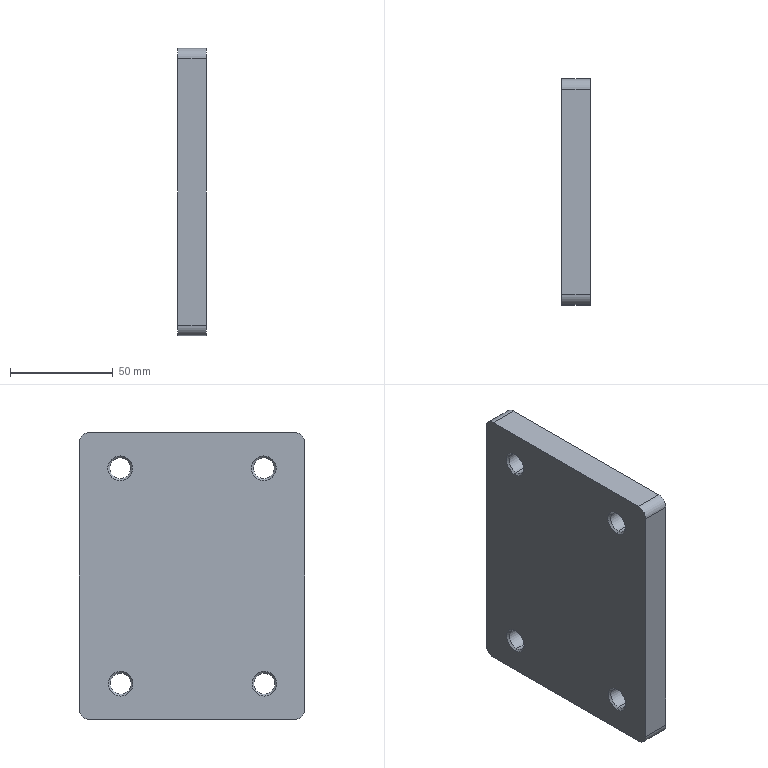Part | SolidWorks | features Extrusion 1, Fillet 1, HoleWzd 1 | 1 solid | 26 faces | box 14 x 110 x 140 mm | volume 210665 mm3 | cylinder 12 | cone 8 | plane 6 | commonest cylinder face diameters 10.2 x8 10 x4
STEP:
#1=CARTESIAN_POINT('',(0.925,34.757,-57.6));
#2=VERTEX_POINT('',#1);
#3=CARTESIAN_POINT('',(0.925,34.757,-47.4));
#4=VERTEX_POINT('',#3);
#5=CARTESIAN_POINT('',(0.925,34.757,-52.5));
#6=DIRECTION('',(-1.,0.,0.));
#7=DIRECTION('',(0.,0.,1.));
#8=AXIS2_PLACEMENT_3D('',#5,#6,#7);
#9=CIRCLE('',#8,5.1);
#10=EDGE_CURVE('',#2,#4,#9,.T.);
#11=ORIENTED_EDGE('',*,*,#10,.F.);
#12=CARTESIAN_POINT('',(0.,34.757,-58.525));
#13=VERTEX_POINT('',#12);
#14=CARTESIAN_POINT('',(0.,34.757,-58.525));
#15=DIRECTION('',(-0.7071,0.,-0.7071));
#16=VECTOR('',#15,1000.);
#17=LINE('',#14,#16);
#18=EDGE_CURVE('',#2,#13,#17,.T.);
#19=ORIENTED_EDGE('',*,*,#18,.T.);
#20=CARTESIAN_POINT('',(0.,34.757,-46.475));
#21=VERTEX_POINT('',#20);
#22=CARTESIAN_POINT('',(0.,34.757,-52.5));
#23=DIRECTION('',(-1.,0.,0.));
#24=DIRECTION('',(0.,0.,1.));
#25=AXIS2_PLACEMENT_3D('',#22,#23,#24);
#26=CIRCLE('',#25,6.025);
#27=EDGE_CURVE('',#13,#21,#26,.T.);
#28=ORIENTED_EDGE('',*,*,#27,.T.);
#29=CARTESIAN_POINT('',(0.,34.757,-46.475));
#30=DIRECTION('',(-0.7071,0.,0.7071));
#31=VECTOR('',#30,1000.);
#32=LINE('',#29,#31);
#33=EDGE_CURVE('',#4,#21,#32,.T.);
#34=ORIENTED_EDGE('',*,*,#33,.F.);
#35=EDGE_LOOP('',(#11,#19,#28,#34));
#36=FACE_OUTER_BOUND('',#35,.T.);
#37=CARTESIAN_POINT('',(0.,34.757,-52.5));
#38=DIRECTION('',(-1.,0.,0.));
#39=DIRECTION('',(0.,0.,1.));
#40=AXIS2_PLACEMENT_3D('',#37,#38,#39);
#41=CONICAL_SURFACE('',#40,6.025,0.7854);
#42=ADVANCED_FACE('',(#36),#41,.F.);
#43=CARTESIAN_POINT('',(14.,34.757,-57.6));
#44=VERTEX_POINT('',#43);
#45=CARTESIAN_POINT('',(14.,34.757,-47.4));
#46=VERTEX_POINT('',#45);
#47=CARTESIAN_POINT('',(14.,34.757,-52.5));
#48=DIRECTION('',(-1.,0.,0.));
#49=DIRECTION('',(0.,0.,1.));
#50=AXIS2_PLACEMENT_3D('',#47,#48,#49);
#51=CIRCLE('',#50,5.1);
#52=EDGE_CURVE('',#44,#46,#51,.T.);
#53=ORIENTED_EDGE('',*,*,#52,.F.);
#54=CARTESIAN_POINT('',(0.,34.757,-57.6));
#55=DIRECTION('',(-1.,0.,0.));
#56=VECTOR('',#55,1000.);
#57=LINE('',#54,#56);
#58=EDGE_CURVE('',#44,#2,#57,.T.);
#59=ORIENTED_EDGE('',*,*,#58,.T.);
#60=ORIENTED_EDGE('',*,*,#10,.T.);
#61=CARTESIAN_POINT('',(0.,34.757,-47.4));
#62=DIRECTION('',(-1.,0.,0.));
#63=VECTOR('',#62,1000.);
#64=LINE('',#61,#63);
#65=EDGE_CURVE('',#46,#4,#64,.T.);
#66=ORIENTED_EDGE('',*,*,#65,.F.);
#67=EDGE_LOOP('',(#53,#59,#60,#66));
#68=FACE_OUTER_BOUND('',#67,.T.);
#69=CARTESIAN_POINT('',(0.,34.757,-52.5));
#70=DIRECTION('',(-1.,0.,0.));
#71=DIRECTION('',(0.,0.,1.));
#72=AXIS2_PLACEMENT_3D('',#69,#70,#71);
#73=CYLINDRICAL_SURFACE('',#72,5.1);
#74=ADVANCED_FACE('',(#68),#73,.F.);
#75=CARTESIAN_POINT('',(0.925,35.,47.4));
#76=VERTEX_POINT('',#75);
#77=CARTESIAN_POINT('',(0.925,35.,57.6));
#78=VERTEX_POINT('',#77);
#79=CARTESIAN_POINT('',(0.925,35.,52.5));
#80=DIRECTION('',(-1.,0.,0.));
#81=DIRECTION('',(0.,0.,1.));
#82=AXIS2_PLACEMENT_3D('',#79,#80,#81);
#83=CIRCLE('',#82,5.1);
#84=EDGE_CURVE('',#76,#78,#83,.T.);
#85=ORIENTED_EDGE('',*,*,#84,.F.);
#86=CARTESIAN_POINT('',(0.,35.,46.475));
#87=VERTEX_POINT('',#86);
#88=CARTESIAN_POINT('',(0.,35.,46.475));
#89=DIRECTION('',(-0.7071,0.,-0.7071));
#90=VECTOR('',#89,1000.);
#91=LINE('',#88,#90);
#92=EDGE_CURVE('',#76,#87,#91,.T.);
#93=ORIENTED_EDGE('',*,*,#92,.T.);
#94=CARTESIAN_POINT('',(0.,35.,58.525));
#95=VERTEX_POINT('',#94);
#96=CARTESIAN_POINT('',(0.,35.,52.5));
#97=DIRECTION('',(-1.,0.,0.));
#98=DIRECTION('',(0.,0.,1.));
#99=AXIS2_PLACEMENT_3D('',#96,#97,#98);
#100=CIRCLE('',#99,6.025);
#101=EDGE_CURVE('',#87,#95,#100,.T.);
#102=ORIENTED_EDGE('',*,*,#101,.T.);
#103=CARTESIAN_POINT('',(0.,35.,58.525));
#104=DIRECTION('',(-0.7071,0.,0.7071));
#105=VECTOR('',#104,1000.);
#106=LINE('',#103,#105);
#107=EDGE_CURVE('',#78,#95,#106,.T.);
#108=ORIENTED_EDGE('',*,*,#107,.F.);
#109=EDGE_LOOP('',(#85,#93,#102,#108));
#110=FACE_OUTER_BOUND('',#109,.T.);
#111=CARTESIAN_POINT('',(0.,35.,52.5));
#112=DIRECTION('',(-1.,0.,0.));
#113=DIRECTION('',(0.,0.,1.));
#114=AXIS2_PLACEMENT_3D('',#111,#112,#113);
#115=CONICAL_SURFACE('',#114,6.025,0.7854);
#116=ADVANCED_FACE('',(#110),#115,.F.);
#117=CARTESIAN_POINT('',(14.,35.,47.4));
#118=VERTEX_POINT('',#117);
#119=CARTESIAN_POINT('',(14.,35.,57.6));
#120=VERTEX_POINT('',#119);
#121=CARTESIAN_POINT('',(14.,35.,52.5));
#122=DIRECTION('',(-1.,0.,0.));
#123=DIRECTION('',(0.,0.,1.));
#124=AXIS2_PLACEMENT_3D('',#121,#122,#123);
#125=CIRCLE('',#124,5.1);
#126=EDGE_CURVE('',#118,#120,#125,.T.);
#127=ORIENTED_EDGE('',*,*,#126,.F.);
#128=CARTESIAN_POINT('',(0.,35.,47.4));
#129=DIRECTION('',(-1.,0.,0.));
#130=VECTOR('',#129,1000.);
#131=LINE('',#128,#130);
#132=EDGE_CURVE('',#118,#76,#131,.T.);
#133=ORIENTED_EDGE('',*,*,#132,.T.);
#134=ORIENTED_EDGE('',*,*,#84,.T.);
#135=CARTESIAN_POINT('',(0.,35.,57.6));
#136=DIRECTION('',(-1.,0.,0.));
#137=VECTOR('',#136,1000.);
#138=LINE('',#135,#137);
#139=EDGE_CURVE('',#120,#78,#138,.T.);
#140=ORIENTED_EDGE('',*,*,#139,.F.);
#141=EDGE_LOOP('',(#127,#133,#134,#140));
#142=FACE_OUTER_BOUND('',#141,.T.);
#143=CARTESIAN_POINT('',(0.,35.,52.5));
#144=DIRECTION('',(-1.,0.,0.));
#145=DIRECTION('',(0.,0.,1.));
#146=AXIS2_PLACEMENT_3D('',#143,#144,#145);
#147=CYLINDRICAL_SURFACE('',#146,5.1);
#148=ADVANCED_FACE('',(#142),#147,.F.);
#149=CARTESIAN_POINT('',(0.925,-35.,47.4));
#150=VERTEX_POINT('',#149);
#151=CARTESIAN_POINT('',(0.925,-35.,57.6));
#152=VERTEX_POINT('',#151);
#153=CARTESIAN_POINT('',(0.925,-35.,52.5));
#154=DIRECTION('',(-1.,0.,0.));
#155=DIRECTION('',(0.,0.,1.));
#156=AXIS2_PLACEMENT_3D('',#153,#154,#155);
#157=CIRCLE('',#156,5.1);
#158=EDGE_CURVE('',#150,#152,#157,.T.);
#159=ORIENTED_EDGE('',*,*,#158,.F.);
#160=CARTESIAN_POINT('',(0.,-35.,46.475));
#161=VERTEX_POINT('',#160);
#162=CARTESIAN_POINT('',(0.,-35.,46.475));
#163=DIRECTION('',(-0.7071,0.,-0.7071));
#164=VECTOR('',#163,1000.);
#165=LINE('',#162,#164);
#166=EDGE_CURVE('',#150,#161,#165,.T.);
#167=ORIENTED_EDGE('',*,*,#166,.T.);
#168=CARTESIAN_POINT('',(0.,-35.,58.525));
#169=VERTEX_POINT('',#168);
#170=CARTESIAN_POINT('',(0.,-35.,52.5));
#171=DIRECTION('',(-1.,0.,0.));
#172=DIRECTION('',(0.,0.,1.));
#173=AXIS2_PLACEMENT_3D('',#170,#171,#172);
#174=CIRCLE('',#173,6.025);
#175=EDGE_CURVE('',#161,#169,#174,.T.);
#176=ORIENTED_EDGE('',*,*,#175,.T.);
#177=CARTESIAN_POINT('',(0.,-35.,58.525));
#178=DIRECTION('',(-0.7071,0.,0.7071));
#179=VECTOR('',#178,1000.);
#180=LINE('',#177,#179);
#181=EDGE_CURVE('',#152,#169,#180,.T.);
#182=ORIENTED_EDGE('',*,*,#181,.F.);
#183=EDGE_LOOP('',(#159,#167,#176,#182));
#184=FACE_OUTER_BOUND('',#183,.T.);
#185=CARTESIAN_POINT('',(0.,-35.,52.5));
#186=DIRECTION('',(-1.,0.,0.));
#187=DIRECTION('',(0.,0.,1.));
#188=AXIS2_PLACEMENT_3D('',#185,#186,#187);
#189=CONICAL_SURFACE('',#188,6.025,0.7854);
#190=ADVANCED_FACE('',(#184),#189,.F.);
#191=CARTESIAN_POINT('',(14.,-35.,47.4));
#192=VERTEX_POINT('',#191);
#193=CARTESIAN_POINT('',(14.,-35.,57.6));
#194=VERTEX_POINT('',#193);
#195=CARTESIAN_POINT('',(14.,-35.,52.5));
#196=DIRECTION('',(-1.,0.,0.));
#197=DIRECTION('',(0.,0.,1.));
#198=AXIS2_PLACEMENT_3D('',#195,#196,#197);
#199=CIRCLE('',#198,5.1);
#200=EDGE_CURVE('',#192,#194,#199,.T.);
#201=ORIENTED_EDGE('',*,*,#200,.F.);
#202=CARTESIAN_POINT('',(0.,-35.,47.4));
#203=DIRECTION('',(-1.,0.,0.));
#204=VECTOR('',#203,1000.);
#205=LINE('',#202,#204);
#206=EDGE_CURVE('',#192,#150,#205,.T.);
#207=ORIENTED_EDGE('',*,*,#206,.T.);
#208=ORIENTED_EDGE('',*,*,#158,.T.);
#209=CARTESIAN_POINT('',(0.,-35.,57.6));
#210=DIRECTION('',(-1.,0.,0.));
#211=VECTOR('',#210,1000.);
#212=LINE('',#209,#211);
#213=EDGE_CURVE('',#194,#152,#212,.T.);
#214=ORIENTED_EDGE('',*,*,#213,.F.);
#215=EDGE_LOOP('',(#201,#207,#208,#214));
#216=FACE_OUTER_BOUND('',#215,.T.);
#217=CARTESIAN_POINT('',(0.,-35.,52.5));
#218=DIRECTION('',(-1.,0.,0.));
#219=DIRECTION('',(0.,0.,1.));
#220=AXIS2_PLACEMENT_3D('',#217,#218,#219);
#221=CYLINDRICAL_SURFACE('',#220,5.1);
#222=ADVANCED_FACE('',(#216),#221,.F.);
#223=CARTESIAN_POINT('',(0.925,-35.243,-57.6));
#224=VERTEX_POINT('',#223);
#225=CARTESIAN_POINT('',(0.925,-35.243,-47.4));
#226=VERTEX_POINT('',#225);
#227=CARTESIAN_POINT('',(0.925,-35.243,-52.5));
#228=DIRECTION('',(-1.,0.,0.));
#229=DIRECTION('',(0.,0.,1.));
#230=AXIS2_PLACEMENT_3D('',#227,#228,#229);
#231=CIRCLE('',#230,5.1);
#232=EDGE_CURVE('',#224,#226,#231,.T.);
#233=ORIENTED_EDGE('',*,*,#232,.F.);
#234=CARTESIAN_POINT('',(0.,-35.243,-58.525));
#235=VERTEX_POINT('',#234);
#236=CARTESIAN_POINT('',(0.,-35.243,-58.525));
#237=DIRECTION('',(-0.7071,0.,-0.7071));
#238=VECTOR('',#237,1000.);
#239=LINE('',#236,#238);
#240=EDGE_CURVE('',#224,#235,#239,.T.);
#241=ORIENTED_EDGE('',*,*,#240,.T.);
#242=CARTESIAN_POINT('',(0.,-35.243,-46.475));
#243=VERTEX_POINT('',#242);
#244=CARTESIAN_POINT('',(0.,-35.243,-52.5));
#245=DIRECTION('',(-1.,0.,0.));
#246=DIRECTION('',(0.,0.,1.));
#247=AXIS2_PLACEMENT_3D('',#244,#245,#246);
#248=CIRCLE('',#247,6.025);
#249=EDGE_CURVE('',#235,#243,#248,.T.);
#250=ORIENTED_EDGE('',*,*,#249,.T.);
#251=CARTESIAN_POINT('',(0.,-35.243,-46.475));
#252=DIRECTION('',(-0.7071,0.,0.7071));
#253=VECTOR('',#252,1000.);
#254=LINE('',#251,#253);
#255=EDGE_CURVE('',#226,#243,#254,.T.);
#256=ORIENTED_EDGE('',*,*,#255,.F.);
#257=EDGE_LOOP('',(#233,#241,#250,#256));
#258=FACE_OUTER_BOUND('',#257,.T.);
#259=CARTESIAN_POINT('',(0.,-35.243,-52.5));
#260=DIRECTION('',(-1.,0.,0.));
#261=DIRECTION('',(0.,0.,1.));
#262=AXIS2_PLACEMENT_3D('',#259,#260,#261);
#263=CONICAL_SURFACE('',#262,6.025,0.7854);
#264=ADVANCED_FACE('',(#258),#263,.F.);
#265=CARTESIAN_POINT('',(14.,-35.243,-57.6));
#266=VERTEX_POINT('',#265);
#267=CARTESIAN_POINT('',(14.,-35.243,-47.4));
#268=VERTEX_POINT('',#267);
#269=CARTESIAN_POINT('',(14.,-35.243,-52.5));
#270=DIRECTION('',(-1.,0.,0.));
#271=DIRECTION('',(0.,0.,1.));
#272=AXIS2_PLACEMENT_3D('',#269,#270,#271);
#273=CIRCLE('',#272,5.1);
#274=EDGE_CURVE('',#266,#268,#273,.T.);
#275=ORIENTED_EDGE('',*,*,#274,.F.);
#276=CARTESIAN_POINT('',(0.,-35.243,-57.6));
#277=DIRECTION('',(-1.,0.,0.));
#278=VECTOR('',#277,1000.);
#279=LINE('',#276,#278);
#280=EDGE_CURVE('',#266,#224,#279,.T.);
#281=ORIENTED_EDGE('',*,*,#280,.T.);
#282=ORIENTED_EDGE('',*,*,#232,.T.);
#283=CARTESIAN_POINT('',(0.,-35.243,-47.4));
#284=DIRECTION('',(-1.,0.,0.));
#285=VECTOR('',#284,1000.);
#286=LINE('',#283,#285);
#287=EDGE_CURVE('',#268,#226,#286,.T.);
#288=ORIENTED_EDGE('',*,*,#287,.F.);
#289=EDGE_LOOP('',(#275,#281,#282,#288));
#290=FACE_OUTER_BOUND('',#289,.T.);
#291=CARTESIAN_POINT('',(0.,-35.243,-52.5));
#292=DIRECTION('',(-1.,0.,0.));
#293=DIRECTION('',(0.,0.,1.));
#294=AXIS2_PLACEMENT_3D('',#291,#292,#293);
#295=CYLINDRICAL_SURFACE('',#294,5.1);
#296=ADVANCED_FACE('',(#290),#295,.F.);
#297=CARTESIAN_POINT('',(14.,-50.,-70.));
#298=VERTEX_POINT('',#297);
#299=CARTESIAN_POINT('',(14.,50.,-70.));
#300=VERTEX_POINT('',#299);
#301=CARTESIAN_POINT('',(14.,-55.,-70.));
#302=DIRECTION('',(0.,1.,0.));
#303=VECTOR('',#302,1000.);
#304=LINE('',#301,#303);
#305=EDGE_CURVE('',#298,#300,#304,.T.);
#306=ORIENTED_EDGE('',*,*,#305,.F.);
#307=CARTESIAN_POINT('',(0.,-50.,-70.));
#308=VERTEX_POINT('',#307);
#309=CARTESIAN_POINT('',(14.,-50.,-70.));
#310=DIRECTION('',(-1.,0.,0.));
#311=VECTOR('',#310,1000.);
#312=LINE('',#309,#311);
#313=EDGE_CURVE('',#298,#308,#312,.T.);
#314=ORIENTED_EDGE('',*,*,#313,.T.);
#315=CARTESIAN_POINT('',(0.,50.,-70.));
#316=VERTEX_POINT('',#315);
#317=CARTESIAN_POINT('',(0.,-55.,-70.));
#318=DIRECTION('',(0.,1.,0.));
#319=VECTOR('',#318,1000.);
#320=LINE('',#317,#319);
#321=EDGE_CURVE('',#308,#316,#320,.T.);
#322=ORIENTED_EDGE('',*,*,#321,.T.);
#323=CARTESIAN_POINT('',(14.,50.,-70.));
#324=DIRECTION('',(1.,0.,0.));
#325=VECTOR('',#324,1000.);
#326=LINE('',#323,#325);
#327=EDGE_CURVE('',#316,#300,#326,.T.);
#328=ORIENTED_EDGE('',*,*,#327,.T.);
#329=EDGE_LOOP('',(#306,#314,#322,#328));
#330=FACE_OUTER_BOUND('',#329,.T.);
#331=CARTESIAN_POINT('',(14.,-55.,-70.));
#332=DIRECTION('',(0.,0.,1.));
#333=DIRECTION('',(1.,0.,0.));
#334=AXIS2_PLACEMENT_3D('',#331,#332,#333);
#335=PLANE('',#334);
#336=ADVANCED_FACE('',(#330),#335,.F.);
#337=CARTESIAN_POINT('',(14.,55.,-65.));
#338=VERTEX_POINT('',#337);
#339=CARTESIAN_POINT('',(14.,55.,65.));
#340=VERTEX_POINT('',#339);
#341=CARTESIAN_POINT('',(14.,55.,70.));
#342=DIRECTION('',(0.,0.,1.));
#343=VECTOR('',#342,1000.);
#344=LINE('',#341,#343);
#345=EDGE_CURVE('',#338,#340,#344,.T.);
#346=ORIENTED_EDGE('',*,*,#345,.F.);
#347=CARTESIAN_POINT('',(0.,55.,-65.));
#348=VERTEX_POINT('',#347);
#349=CARTESIAN_POINT('',(14.,55.,-65.));
#350=DIRECTION('',(-1.,0.,0.));
#351=VECTOR('',#350,1000.);
#352=LINE('',#349,#351);
#353=EDGE_CURVE('',#338,#348,#352,.T.);
#354=ORIENTED_EDGE('',*,*,#353,.T.);
#355=CARTESIAN_POINT('',(0.,55.,65.));
#356=VERTEX_POINT('',#355);
#357=CARTESIAN_POINT('',(0.,55.,70.));
#358=DIRECTION('',(0.,0.,1.));
#359=VECTOR('',#358,1000.);
#360=LINE('',#357,#359);
#361=EDGE_CURVE('',#348,#356,#360,.T.);
#362=ORIENTED_EDGE('',*,*,#361,.T.);
#363=CARTESIAN_POINT('',(14.,55.,65.));
#364=DIRECTION('',(1.,0.,0.));
#365=VECTOR('',#364,1000.);
#366=LINE('',#363,#365);
#367=EDGE_CURVE('',#356,#340,#366,.T.);
#368=ORIENTED_EDGE('',*,*,#367,.T.);
#369=EDGE_LOOP('',(#346,#354,#362,#368));
#370=FACE_OUTER_BOUND('',#369,.T.);
#371=CARTESIAN_POINT('',(14.,55.,70.));
#372=DIRECTION('',(0.,-1.,0.));
#373=DIRECTION('',(0.,0.,-1.));
#374=AXIS2_PLACEMENT_3D('',#371,#372,#373);
#375=PLANE('',#374);
#376=ADVANCED_FACE('',(#370),#375,.F.);
#377=CARTESIAN_POINT('',(0.,50.,70.));
#378=VERTEX_POINT('',#377);
#379=CARTESIAN_POINT('',(0.,-50.,70.));
#380=VERTEX_POINT('',#379);
#381=CARTESIAN_POINT('',(0.,-55.,70.));
#382=DIRECTION('',(0.,-1.,0.));
#383=VECTOR('',#382,1000.);
#384=LINE('',#381,#383);
#385=EDGE_CURVE('',#378,#380,#384,.T.);
#386=ORIENTED_EDGE('',*,*,#385,.T.);
#387=CARTESIAN_POINT('',(14.,-50.,70.));
#388=VERTEX_POINT('',#387);
#389=CARTESIAN_POINT('',(14.,-50.,70.));
#390=DIRECTION('',(1.,0.,0.));
#391=VECTOR('',#390,1000.);
#392=LINE('',#389,#391);
#393=EDGE_CURVE('',#380,#388,#392,.T.);
#394=ORIENTED_EDGE('',*,*,#393,.T.);
#395=CARTESIAN_POINT('',(14.,50.,70.));
#396=VERTEX_POINT('',#395);
#397=CARTESIAN_POINT('',(14.,-55.,70.));
#398=DIRECTION('',(0.,-1.,0.));
#399=VECTOR('',#398,1000.);
#400=LINE('',#397,#399);
#401=EDGE_CURVE('',#396,#388,#400,.T.);
#402=ORIENTED_EDGE('',*,*,#401,.F.);
#403=CARTESIAN_POINT('',(14.,50.,70.));
#404=DIRECTION('',(-1.,0.,0.));
#405=VECTOR('',#404,1000.);
#406=LINE('',#403,#405);
#407=EDGE_CURVE('',#396,#378,#406,.T.);
#408=ORIENTED_EDGE('',*,*,#407,.T.);
#409=EDGE_LOOP('',(#386,#394,#402,#408));
#410=FACE_OUTER_BOUND('',#409,.T.);
#411=CARTESIAN_POINT('',(14.,-55.,70.));
#412=DIRECTION('',(0.,0.,-1.));
#413=DIRECTION('',(-1.,0.,0.));
#414=AXIS2_PLACEMENT_3D('',#411,#412,#413);
#415=PLANE('',#414);
#416=ADVANCED_FACE('',(#410),#415,.F.);
#417=CARTESIAN_POINT('',(0.,-55.,65.));
#418=VERTEX_POINT('',#417);
#419=CARTESIAN_POINT('',(0.,-55.,-65.));
#420=VERTEX_POINT('',#419);
#421=CARTESIAN_POINT('',(0.,-55.,70.));
#422=DIRECTION('',(0.,0.,-1.));
#423=VECTOR('',#422,1000.);
#424=LINE('',#421,#423);
#425=EDGE_CURVE('',#418,#420,#424,.T.);
#426=ORIENTED_EDGE('',*,*,#425,.T.);
#427=CARTESIAN_POINT('',(14.,-55.,-65.));
#428=VERTEX_POINT('',#427);
#429=CARTESIAN_POINT('',(14.,-55.,-65.));
#430=DIRECTION('',(1.,0.,0.));
#431=VECTOR('',#430,1000.);
#432=LINE('',#429,#431);
#433=EDGE_CURVE('',#420,#428,#432,.T.);
#434=ORIENTED_EDGE('',*,*,#433,.T.);
#435=CARTESIAN_POINT('',(14.,-55.,65.));
#436=VERTEX_POINT('',#435);
#437=CARTESIAN_POINT('',(14.,-55.,70.));
#438=DIRECTION('',(0.,0.,-1.));
#439=VECTOR('',#438,1000.);
#440=LINE('',#437,#439);
#441=EDGE_CURVE('',#436,#428,#440,.T.);
#442=ORIENTED_EDGE('',*,*,#441,.F.);
#443=CARTESIAN_POINT('',(14.,-55.,65.));
#444=DIRECTION('',(-1.,0.,0.));
#445=VECTOR('',#444,1000.);
#446=LINE('',#443,#445);
#447=EDGE_CURVE('',#436,#418,#446,.T.);
#448=ORIENTED_EDGE('',*,*,#447,.T.);
#449=EDGE_LOOP('',(#426,#434,#442,#448));
#450=FACE_OUTER_BOUND('',#449,.T.);
#451=CARTESIAN_POINT('',(14.,-55.,70.));
#452=DIRECTION('',(0.,1.,0.));
#453=DIRECTION('',(0.,0.,1.));
#454=AXIS2_PLACEMENT_3D('',#451,#452,#453);
#455=PLANE('',#454);
#456=ADVANCED_FACE('',(#450),#455,.F.);
#457=CARTESIAN_POINT('',(14.,34.757,-52.5));
#458=DIRECTION('',(-1.,0.,0.));
#459=DIRECTION('',(0.,0.,1.));
#460=AXIS2_PLACEMENT_3D('',#457,#458,#459);
#461=CIRCLE('',#460,5.1);
#462=EDGE_CURVE('',#46,#44,#461,.T.);
#463=ORIENTED_EDGE('',*,*,#462,.T.);
#464=ORIENTED_EDGE('',*,*,#52,.T.);
#465=EDGE_LOOP('',(#463,#464));
#466=FACE_BOUND('',#465,.T.);
#467=CARTESIAN_POINT('',(14.,35.,52.5));
#468=DIRECTION('',(-1.,0.,0.));
#469=DIRECTION('',(0.,0.,1.));
#470=AXIS2_PLACEMENT_3D('',#467,#468,#469);
#471=CIRCLE('',#470,5.1);
#472=EDGE_CURVE('',#120,#118,#471,.T.);
#473=ORIENTED_EDGE('',*,*,#472,.T.);
#474=ORIENTED_EDGE('',*,*,#126,.T.);
#475=EDGE_LOOP('',(#473,#474));
#476=FACE_BOUND('',#475,.T.);
#477=CARTESIAN_POINT('',(14.,-35.,52.5));
#478=DIRECTION('',(-1.,0.,0.));
#479=DIRECTION('',(0.,0.,1.));
#480=AXIS2_PLACEMENT_3D('',#477,#478,#479);
#481=CIRCLE('',#480,5.1);
#482=EDGE_CURVE('',#194,#192,#481,.T.);
#483=ORIENTED_EDGE('',*,*,#482,.T.);
#484=ORIENTED_EDGE('',*,*,#200,.T.);
#485=EDGE_LOOP('',(#483,#484));
#486=FACE_BOUND('',#485,.T.);
#487=CARTESIAN_POINT('',(14.,-35.243,-52.5));
#488=DIRECTION('',(-1.,0.,0.));
#489=DIRECTION('',(0.,0.,1.));
#490=AXIS2_PLACEMENT_3D('',#487,#488,#489);
#491=CIRCLE('',#490,5.1);
#492=EDGE_CURVE('',#268,#266,#491,.T.);
#493=ORIENTED_EDGE('',*,*,#492,.T.);
#494=ORIENTED_EDGE('',*,*,#274,.T.);
#495=EDGE_LOOP('',(#493,#494));
#496=FACE_BOUND('',#495,.T.);
#497=ORIENTED_EDGE('',*,*,#441,.T.);
#498=CARTESIAN_POINT('',(14.,-50.,-65.));
#499=DIRECTION('',(1.,0.,0.));
#500=DIRECTION('',(0.,0.,1.));
#501=AXIS2_PLACEMENT_3D('',#498,#499,#500);
#502=CIRCLE('',#501,5.);
#503=EDGE_CURVE('',#428,#298,#502,.T.);
#504=ORIENTED_EDGE('',*,*,#503,.T.);
#505=ORIENTED_EDGE('',*,*,#305,.T.);
#506=CARTESIAN_POINT('',(14.,50.,-65.));
#507=DIRECTION('',(1.,0.,0.));
#508=DIRECTION('',(0.,0.,1.));
#509=AXIS2_PLACEMENT_3D('',#506,#507,#508);
#510=CIRCLE('',#509,5.);
#511=EDGE_CURVE('',#300,#338,#510,.T.);
#512=ORIENTED_EDGE('',*,*,#511,.T.);
#513=ORIENTED_EDGE('',*,*,#345,.T.);
#514=CARTESIAN_POINT('',(14.,50.,65.));
#515=DIRECTION('',(1.,0.,0.));
#516=DIRECTION('',(0.,0.,1.));
#517=AXIS2_PLACEMENT_3D('',#514,#515,#516);
#518=CIRCLE('',#517,5.);
#519=EDGE_CURVE('',#340,#396,#518,.T.);
#520=ORIENTED_EDGE('',*,*,#519,.T.);
#521=ORIENTED_EDGE('',*,*,#401,.T.);
#522=CARTESIAN_POINT('',(14.,-50.,65.));
#523=DIRECTION('',(1.,0.,0.));
#524=DIRECTION('',(0.,0.,1.));
#525=AXIS2_PLACEMENT_3D('',#522,#523,#524);
#526=CIRCLE('',#525,5.);
#527=EDGE_CURVE('',#388,#436,#526,.T.);
#528=ORIENTED_EDGE('',*,*,#527,.T.);
#529=EDGE_LOOP('',(#497,#504,#505,#512,#513,#520,#521,#528));
#530=FACE_OUTER_BOUND('',#529,.T.);
#531=CARTESIAN_POINT('',(14.,0.,0.));
#532=DIRECTION('',(-1.,0.,0.));
#533=DIRECTION('',(0.,0.,1.));
#534=AXIS2_PLACEMENT_3D('',#531,#532,#533);
#535=PLANE('',#534);
#536=ADVANCED_FACE('',(#466,#476,#486,#496,#530),#535,.F.);
#537=CARTESIAN_POINT('',(0.,34.757,-52.5));
#538=DIRECTION('',(-1.,0.,0.));
#539=DIRECTION('',(0.,0.,1.));
#540=AXIS2_PLACEMENT_3D('',#537,#538,#539);
#541=CIRCLE('',#540,6.025);
#542=EDGE_CURVE('',#21,#13,#541,.T.);
#543=ORIENTED_EDGE('',*,*,#542,.F.);
#544=ORIENTED_EDGE('',*,*,#27,.F.);
#545=EDGE_LOOP('',(#543,#544));
#546=FACE_BOUND('',#545,.T.);
#547=CARTESIAN_POINT('',(0.,35.,52.5));
#548=DIRECTION('',(-1.,0.,0.));
#549=DIRECTION('',(0.,0.,1.));
#550=AXIS2_PLACEMENT_3D('',#547,#548,#549);
#551=CIRCLE('',#550,6.025);
#552=EDGE_CURVE('',#95,#87,#551,.T.);
#553=ORIENTED_EDGE('',*,*,#552,.F.);
#554=ORIENTED_EDGE('',*,*,#101,.F.);
#555=EDGE_LOOP('',(#553,#554));
#556=FACE_BOUND('',#555,.T.);
#557=CARTESIAN_POINT('',(0.,-35.,52.5));
#558=DIRECTION('',(-1.,0.,0.));
#559=DIRECTION('',(0.,0.,1.));
#560=AXIS2_PLACEMENT_3D('',#557,#558,#559);
#561=CIRCLE('',#560,6.025);
#562=EDGE_CURVE('',#169,#161,#561,.T.);
#563=ORIENTED_EDGE('',*,*,#562,.F.);
#564=ORIENTED_EDGE('',*,*,#175,.F.);
#565=EDGE_LOOP('',(#563,#564));
#566=FACE_BOUND('',#565,.T.);
#567=CARTESIAN_POINT('',(0.,-35.243,-52.5));
#568=DIRECTION('',(-1.,0.,0.));
#569=DIRECTION('',(0.,0.,1.));
#570=AXIS2_PLACEMENT_3D('',#567,#568,#569);
#571=CIRCLE('',#570,6.025);
#572=EDGE_CURVE('',#243,#235,#571,.T.);
#573=ORIENTED_EDGE('',*,*,#572,.F.);
#574=ORIENTED_EDGE('',*,*,#249,.F.);
#575=EDGE_LOOP('',(#573,#574));
#576=FACE_BOUND('',#575,.T.);
#577=ORIENTED_EDGE('',*,*,#321,.F.);
#578=CARTESIAN_POINT('',(0.,-50.,-65.));
#579=DIRECTION('',(-1.,0.,0.));
#580=DIRECTION('',(0.,0.,1.));
#581=AXIS2_PLACEMENT_3D('',#578,#579,#580);
#582=CIRCLE('',#581,5.);
#583=EDGE_CURVE('',#308,#420,#582,.T.);
#584=ORIENTED_EDGE('',*,*,#583,.T.);
#585=ORIENTED_EDGE('',*,*,#425,.F.);
#586=CARTESIAN_POINT('',(0.,-50.,65.));
#587=DIRECTION('',(-1.,0.,0.));
#588=DIRECTION('',(0.,0.,1.));
#589=AXIS2_PLACEMENT_3D('',#586,#587,#588);
#590=CIRCLE('',#589,5.);
#591=EDGE_CURVE('',#418,#380,#590,.T.);
#592=ORIENTED_EDGE('',*,*,#591,.T.);
#593=ORIENTED_EDGE('',*,*,#385,.F.);
#594=CARTESIAN_POINT('',(0.,50.,65.));
#595=DIRECTION('',(-1.,0.,0.));
#596=DIRECTION('',(0.,0.,1.));
#597=AXIS2_PLACEMENT_3D('',#594,#595,#596);
#598=CIRCLE('',#597,5.);
#599=EDGE_CURVE('',#378,#356,#598,.T.);
#600=ORIENTED_EDGE('',*,*,#599,.T.);
#601=ORIENTED_EDGE('',*,*,#361,.F.);
#602=CARTESIAN_POINT('',(0.,50.,-65.));
#603=DIRECTION('',(-1.,0.,0.));
#604=DIRECTION('',(0.,0.,1.));
#605=AXIS2_PLACEMENT_3D('',#602,#603,#604);
#606=CIRCLE('',#605,5.);
#607=EDGE_CURVE('',#348,#316,#606,.T.);
#608=ORIENTED_EDGE('',*,*,#607,.T.);
#609=EDGE_LOOP('',(#577,#584,#585,#592,#593,#600,#601,#608));
#610=FACE_OUTER_BOUND('',#609,.T.);
#611=CARTESIAN_POINT('',(0.,0.,0.));
#612=DIRECTION('',(-1.,0.,0.));
#613=DIRECTION('',(0.,0.,1.));
#614=AXIS2_PLACEMENT_3D('',#611,#612,#613);
#615=PLANE('',#614);
#616=ADVANCED_FACE('',(#546,#556,#566,#576,#610),#615,.T.);
#617=ORIENTED_EDGE('',*,*,#503,.F.);
#618=ORIENTED_EDGE('',*,*,#433,.F.);
#619=ORIENTED_EDGE('',*,*,#583,.F.);
#620=ORIENTED_EDGE('',*,*,#313,.F.);
#621=EDGE_LOOP('',(#617,#618,#619,#620));
#622=FACE_OUTER_BOUND('',#621,.T.);
#623=CARTESIAN_POINT('',(14.,-50.,-65.));
#624=DIRECTION('',(-1.,0.,0.));
#625=DIRECTION('',(0.,0.,1.));
#626=AXIS2_PLACEMENT_3D('',#623,#624,#625);
#627=CYLINDRICAL_SURFACE('',#626,5.);
#628=ADVANCED_FACE('',(#622),#627,.T.);
#629=ORIENTED_EDGE('',*,*,#511,.F.);
#630=ORIENTED_EDGE('',*,*,#327,.F.);
#631=ORIENTED_EDGE('',*,*,#607,.F.);
#632=ORIENTED_EDGE('',*,*,#353,.F.);
#633=EDGE_LOOP('',(#629,#630,#631,#632));
#634=FACE_OUTER_BOUND('',#633,.T.);
#635=CARTESIAN_POINT('',(14.,50.,-65.));
#636=DIRECTION('',(-1.,0.,0.));
#637=DIRECTION('',(0.,0.,1.));
#638=AXIS2_PLACEMENT_3D('',#635,#636,#637);
#639=CYLINDRICAL_SURFACE('',#638,5.);
#640=ADVANCED_FACE('',(#634),#639,.T.);
#641=ORIENTED_EDGE('',*,*,#527,.F.);
#642=ORIENTED_EDGE('',*,*,#393,.F.);
#643=ORIENTED_EDGE('',*,*,#591,.F.);
#644=ORIENTED_EDGE('',*,*,#447,.F.);
#645=EDGE_LOOP('',(#641,#642,#643,#644));
#646=FACE_OUTER_BOUND('',#645,.T.);
#647=CARTESIAN_POINT('',(14.,-50.,65.));
#648=DIRECTION('',(-1.,0.,0.));
#649=DIRECTION('',(0.,0.,1.));
#650=AXIS2_PLACEMENT_3D('',#647,#648,#649);
#651=CYLINDRICAL_SURFACE('',#650,5.);
#652=ADVANCED_FACE('',(#646),#651,.T.);
#653=ORIENTED_EDGE('',*,*,#519,.F.);
#654=ORIENTED_EDGE('',*,*,#367,.F.);
#655=ORIENTED_EDGE('',*,*,#599,.F.);
#656=ORIENTED_EDGE('',*,*,#407,.F.);
#657=EDGE_LOOP('',(#653,#654,#655,#656));
#658=FACE_OUTER_BOUND('',#657,.T.);
#659=CARTESIAN_POINT('',(14.,50.,65.));
#660=DIRECTION('',(-1.,0.,0.));
#661=DIRECTION('',(0.,0.,1.));
#662=AXIS2_PLACEMENT_3D('',#659,#660,#661);
#663=CYLINDRICAL_SURFACE('',#662,5.);
#664=ADVANCED_FACE('',(#658),#663,.T.);
#665=ORIENTED_EDGE('',*,*,#280,.F.);
#666=ORIENTED_EDGE('',*,*,#492,.F.);
#667=ORIENTED_EDGE('',*,*,#287,.T.);
#668=CARTESIAN_POINT('',(0.925,-35.243,-52.5));
#669=DIRECTION('',(-1.,0.,0.));
#670=DIRECTION('',(0.,0.,1.));
#671=AXIS2_PLACEMENT_3D('',#668,#669,#670);
#672=CIRCLE('',#671,5.1);
#673=EDGE_CURVE('',#226,#224,#672,.T.);
#674=ORIENTED_EDGE('',*,*,#673,.T.);
#675=EDGE_LOOP('',(#665,#666,#667,#674));
#676=FACE_OUTER_BOUND('',#675,.T.);
#677=CARTESIAN_POINT('',(0.,-35.243,-52.5));
#678=DIRECTION('',(-1.,0.,0.));
#679=DIRECTION('',(0.,0.,1.));
#680=AXIS2_PLACEMENT_3D('',#677,#678,#679);
#681=CYLINDRICAL_SURFACE('',#680,5.1);
#682=ADVANCED_FACE('',(#676),#681,.F.);
#683=ORIENTED_EDGE('',*,*,#240,.F.);
#684=ORIENTED_EDGE('',*,*,#673,.F.);
#685=ORIENTED_EDGE('',*,*,#255,.T.);
#686=ORIENTED_EDGE('',*,*,#572,.T.);
#687=EDGE_LOOP('',(#683,#684,#685,#686));
#688=FACE_OUTER_BOUND('',#687,.T.);
#689=CARTESIAN_POINT('',(0.,-35.243,-52.5));
#690=DIRECTION('',(-1.,0.,0.));
#691=DIRECTION('',(0.,0.,1.));
#692=AXIS2_PLACEMENT_3D('',#689,#690,#691);
#693=CONICAL_SURFACE('',#692,6.025,0.7854);
#694=ADVANCED_FACE('',(#688),#693,.F.);
#695=ORIENTED_EDGE('',*,*,#206,.F.);
#696=ORIENTED_EDGE('',*,*,#482,.F.);
#697=ORIENTED_EDGE('',*,*,#213,.T.);
#698=CARTESIAN_POINT('',(0.925,-35.,52.5));
#699=DIRECTION('',(-1.,0.,0.));
#700=DIRECTION('',(0.,0.,1.));
#701=AXIS2_PLACEMENT_3D('',#698,#699,#700);
#702=CIRCLE('',#701,5.1);
#703=EDGE_CURVE('',#152,#150,#702,.T.);
#704=ORIENTED_EDGE('',*,*,#703,.T.);
#705=EDGE_LOOP('',(#695,#696,#697,#704));
#706=FACE_OUTER_BOUND('',#705,.T.);
#707=CARTESIAN_POINT('',(0.,-35.,52.5));
#708=DIRECTION('',(-1.,0.,0.));
#709=DIRECTION('',(0.,0.,1.));
#710=AXIS2_PLACEMENT_3D('',#707,#708,#709);
#711=CYLINDRICAL_SURFACE('',#710,5.1);
#712=ADVANCED_FACE('',(#706),#711,.F.);
#713=ORIENTED_EDGE('',*,*,#166,.F.);
#714=ORIENTED_EDGE('',*,*,#703,.F.);
#715=ORIENTED_EDGE('',*,*,#181,.T.);
#716=ORIENTED_EDGE('',*,*,#562,.T.);
#717=EDGE_LOOP('',(#713,#714,#715,#716));
#718=FACE_OUTER_BOUND('',#717,.T.);
#719=CARTESIAN_POINT('',(0.,-35.,52.5));
#720=DIRECTION('',(-1.,0.,0.));
#721=DIRECTION('',(0.,0.,1.));
#722=AXIS2_PLACEMENT_3D('',#719,#720,#721);
#723=CONICAL_SURFACE('',#722,6.025,0.7854);
#724=ADVANCED_FACE('',(#718),#723,.F.);
#725=ORIENTED_EDGE('',*,*,#132,.F.);
#726=ORIENTED_EDGE('',*,*,#472,.F.);
#727=ORIENTED_EDGE('',*,*,#139,.T.);
#728=CARTESIAN_POINT('',(0.925,35.,52.5));
#729=DIRECTION('',(-1.,0.,0.));
#730=DIRECTION('',(0.,0.,1.));
#731=AXIS2_PLACEMENT_3D('',#728,#729,#730);
#732=CIRCLE('',#731,5.1);
#733=EDGE_CURVE('',#78,#76,#732,.T.);
#734=ORIENTED_EDGE('',*,*,#733,.T.);
#735=EDGE_LOOP('',(#725,#726,#727,#734));
#736=FACE_OUTER_BOUND('',#735,.T.);
#737=CARTESIAN_POINT('',(0.,35.,52.5));
#738=DIRECTION('',(-1.,0.,0.));
#739=DIRECTION('',(0.,0.,1.));
#740=AXIS2_PLACEMENT_3D('',#737,#738,#739);
#741=CYLINDRICAL_SURFACE('',#740,5.1);
#742=ADVANCED_FACE('',(#736),#741,.F.);
#743=ORIENTED_EDGE('',*,*,#92,.F.);
#744=ORIENTED_EDGE('',*,*,#733,.F.);
#745=ORIENTED_EDGE('',*,*,#107,.T.);
#746=ORIENTED_EDGE('',*,*,#552,.T.);
#747=EDGE_LOOP('',(#743,#744,#745,#746));
#748=FACE_OUTER_BOUND('',#747,.T.);
#749=CARTESIAN_POINT('',(0.,35.,52.5));
#750=DIRECTION('',(-1.,0.,0.));
#751=DIRECTION('',(0.,0.,1.));
#752=AXIS2_PLACEMENT_3D('',#749,#750,#751);
#753=CONICAL_SURFACE('',#752,6.025,0.7854);
#754=ADVANCED_FACE('',(#748),#753,.F.);
#755=ORIENTED_EDGE('',*,*,#58,.F.);
#756=ORIENTED_EDGE('',*,*,#462,.F.);
#757=ORIENTED_EDGE('',*,*,#65,.T.);
#758=CARTESIAN_POINT('',(0.925,34.757,-52.5));
#759=DIRECTION('',(-1.,0.,0.));
#760=DIRECTION('',(0.,0.,1.));
#761=AXIS2_PLACEMENT_3D('',#758,#759,#760);
#762=CIRCLE('',#761,5.1);
#763=EDGE_CURVE('',#4,#2,#762,.T.);
#764=ORIENTED_EDGE('',*,*,#763,.T.);
#765=EDGE_LOOP('',(#755,#756,#757,#764));
#766=FACE_OUTER_BOUND('',#765,.T.);
#767=CARTESIAN_POINT('',(0.,34.757,-52.5));
#768=DIRECTION('',(-1.,0.,0.));
#769=DIRECTION('',(0.,0.,1.));
#770=AXIS2_PLACEMENT_3D('',#767,#768,#769);
#771=CYLINDRICAL_SURFACE('',#770,5.1);
#772=ADVANCED_FACE('',(#766),#771,.F.);
#773=ORIENTED_EDGE('',*,*,#18,.F.);
#774=ORIENTED_EDGE('',*,*,#763,.F.);
#775=ORIENTED_EDGE('',*,*,#33,.T.);
#776=ORIENTED_EDGE('',*,*,#542,.T.);
#777=EDGE_LOOP('',(#773,#774,#775,#776));
#778=FACE_OUTER_BOUND('',#777,.T.);
#779=CARTESIAN_POINT('',(0.,34.757,-52.5));
#780=DIRECTION('',(-1.,0.,0.));
#781=DIRECTION('',(0.,0.,1.));
#782=AXIS2_PLACEMENT_3D('',#779,#780,#781);
#783=CONICAL_SURFACE('',#782,6.025,0.7854);
#784=ADVANCED_FACE('',(#778),#783,.F.);
#785=CLOSED_SHELL('',(#42,#74,#116,#148,#190,#222,#264,#296,#336,#376,#416,#456,#536,#616,#628,#640,#652,#664,#682,#694,#712,#724,#742,#754,#772,#784));
#786=MANIFOLD_SOLID_BREP('',#785);
#787=CARTESIAN_POINT('',(0.,0.,0.));
#788=DIRECTION('',(0.,0.,1.));
#789=DIRECTION('',(1.,0.,0.));
#790=AXIS2_PLACEMENT_3D('',#787,#788,#789);
#791=(LENGTH_UNIT()NAMED_UNIT(*)SI_UNIT(.MILLI.,.METRE.));
#792=UNCERTAINTY_MEASURE_WITH_UNIT(LENGTH_MEASURE(0.00001),#791,'','');
#793=(NAMED_UNIT(*)PLANE_ANGLE_UNIT()SI_UNIT($,.RADIAN.));
#794=(NAMED_UNIT(*)SI_UNIT($,.STERADIAN.)SOLID_ANGLE_UNIT());
#795=(GEOMETRIC_REPRESENTATION_CONTEXT(3)GLOBAL_UNCERTAINTY_ASSIGNED_CONTEXT((#792))GLOBAL_UNIT_ASSIGNED_CONTEXT((#791,#793,#794))REPRESENTATION_CONTEXT('',''));
#796=ADVANCED_BREP_SHAPE_REPRESENTATION('',(#786,#790),#795);